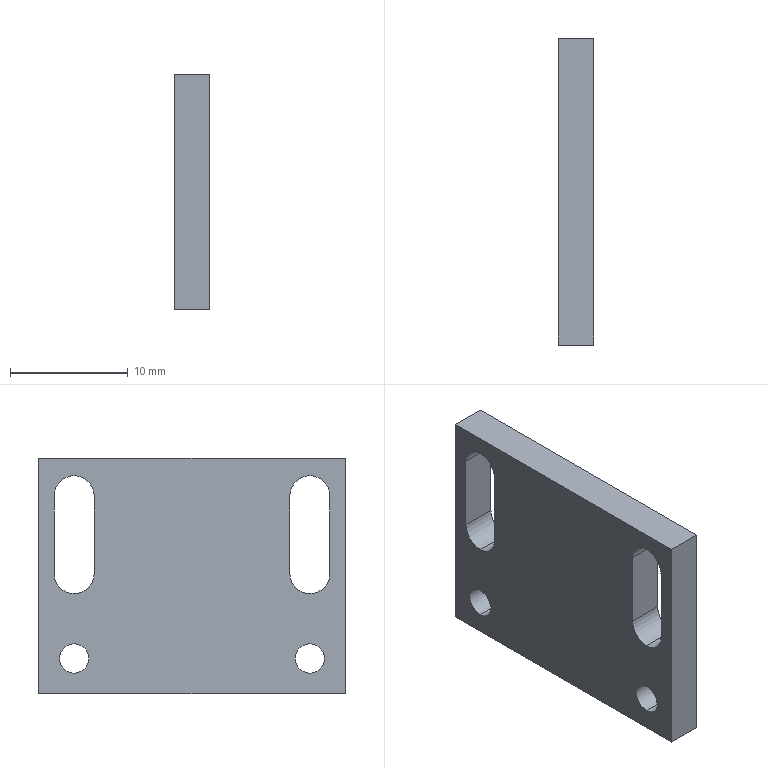Part | NX | features BREP 1 | 1 solid | 20 faces | box 3 x 26 x 20 mm | volume 1341 mm3 | plane 10 | cylinder 10 | commonest cylinder face diameters 3.4 x6 2.5 x4
STEP:
#1=CARTESIAN_POINT('',(3.,11.7,6.8));
#2=VERTEX_POINT('',#1);
#3=CARTESIAN_POINT('',(0.,11.7,6.8));
#4=VERTEX_POINT('',#3);
#5=CARTESIAN_POINT('',(0.,11.7,6.8));
#6=DIRECTION('',(-1.,0.,0.));
#7=VECTOR('',#6,1000.);
#8=LINE('',#5,#7);
#9=EDGE_CURVE('',#2,#4,#8,.T.);
#10=ORIENTED_EDGE('',*,*,#9,.T.);
#11=CARTESIAN_POINT('',(0.,11.7,0.2));
#12=VERTEX_POINT('',#11);
#13=CARTESIAN_POINT('',(0.,11.7,0.2));
#14=DIRECTION('',(0.,0.,1.));
#15=VECTOR('',#14,1000.);
#16=LINE('',#13,#15);
#17=EDGE_CURVE('',#12,#4,#16,.T.);
#18=ORIENTED_EDGE('',*,*,#17,.F.);
#19=CARTESIAN_POINT('',(3.,11.7,0.2));
#20=VERTEX_POINT('',#19);
#21=CARTESIAN_POINT('',(0.,11.7,0.2));
#22=DIRECTION('',(-1.,0.,0.));
#23=VECTOR('',#22,1000.);
#24=LINE('',#21,#23);
#25=EDGE_CURVE('',#20,#12,#24,.T.);
#26=ORIENTED_EDGE('',*,*,#25,.F.);
#27=CARTESIAN_POINT('',(3.,11.7,0.2));
#28=DIRECTION('',(0.,0.,1.));
#29=VECTOR('',#28,1000.);
#30=LINE('',#27,#29);
#31=EDGE_CURVE('',#20,#2,#30,.T.);
#32=ORIENTED_EDGE('',*,*,#31,.T.);
#33=EDGE_LOOP('',(#10,#18,#26,#32));
#34=FACE_BOUND('',#33,.T.);
#35=CARTESIAN_POINT('',(0.,11.7,0.2));
#36=DIRECTION('',(0.,1.,0.));
#37=DIRECTION('',(-1.,0.,0.));
#38=AXIS2_PLACEMENT_3D('',#35,#36,#37);
#39=PLANE('',#38);
#40=ADVANCED_FACE('',(#34),#39,.F.);
#41=CARTESIAN_POINT('',(0.,8.3,6.8));
#42=VERTEX_POINT('',#41);
#43=CARTESIAN_POINT('',(3.,8.3,6.8));
#44=VERTEX_POINT('',#43);
#45=CARTESIAN_POINT('',(3.,8.3,6.8));
#46=DIRECTION('',(1.,0.,0.));
#47=VECTOR('',#46,1000.);
#48=LINE('',#45,#47);
#49=EDGE_CURVE('',#42,#44,#48,.T.);
#50=ORIENTED_EDGE('',*,*,#49,.T.);
#51=CARTESIAN_POINT('',(3.,8.3,0.2));
#52=VERTEX_POINT('',#51);
#53=CARTESIAN_POINT('',(3.,8.3,0.2));
#54=DIRECTION('',(0.,0.,1.));
#55=VECTOR('',#54,1000.);
#56=LINE('',#53,#55);
#57=EDGE_CURVE('',#52,#44,#56,.T.);
#58=ORIENTED_EDGE('',*,*,#57,.F.);
#59=CARTESIAN_POINT('',(0.,8.3,0.2));
#60=VERTEX_POINT('',#59);
#61=CARTESIAN_POINT('',(3.,8.3,0.2));
#62=DIRECTION('',(-1.,0.,0.));
#63=VECTOR('',#62,1000.);
#64=LINE('',#61,#63);
#65=EDGE_CURVE('',#52,#60,#64,.T.);
#66=ORIENTED_EDGE('',*,*,#65,.T.);
#67=CARTESIAN_POINT('',(0.,8.3,0.2));
#68=DIRECTION('',(0.,0.,1.));
#69=VECTOR('',#68,1000.);
#70=LINE('',#67,#69);
#71=EDGE_CURVE('',#60,#42,#70,.T.);
#72=ORIENTED_EDGE('',*,*,#71,.T.);
#73=EDGE_LOOP('',(#50,#58,#66,#72));
#74=FACE_BOUND('',#73,.T.);
#75=CARTESIAN_POINT('',(3.,8.3,0.2));
#76=DIRECTION('',(0.,-1.,0.));
#77=DIRECTION('',(0.,0.,-1.));
#78=AXIS2_PLACEMENT_3D('',#75,#76,#77);
#79=PLANE('',#78);
#80=ADVANCED_FACE('',(#74),#79,.F.);
#81=CARTESIAN_POINT('',(0.,10.,-1.5));
#82=VERTEX_POINT('',#81);
#83=CARTESIAN_POINT('',(3.,10.,-1.5));
#84=VERTEX_POINT('',#83);
#85=CARTESIAN_POINT('',(3.,10.,-1.5));
#86=DIRECTION('',(1.,0.,0.));
#87=VECTOR('',#86,1000.);
#88=LINE('',#85,#87);
#89=EDGE_CURVE('',#82,#84,#88,.T.);
#90=ORIENTED_EDGE('',*,*,#89,.F.);
#91=CARTESIAN_POINT('',(0.,10.,0.2));
#92=DIRECTION('',(1.,0.,0.));
#93=DIRECTION('',(0.,0.,-1.));
#94=AXIS2_PLACEMENT_3D('',#91,#92,#93);
#95=CIRCLE('',#94,1.7);
#96=EDGE_CURVE('',#60,#82,#95,.T.);
#97=ORIENTED_EDGE('',*,*,#96,.F.);
#98=ORIENTED_EDGE('',*,*,#65,.F.);
#99=CARTESIAN_POINT('',(3.,10.,0.2));
#100=DIRECTION('',(1.,0.,0.));
#101=DIRECTION('',(0.,0.,-1.));
#102=AXIS2_PLACEMENT_3D('',#99,#100,#101);
#103=CIRCLE('',#102,1.7);
#104=EDGE_CURVE('',#52,#84,#103,.T.);
#105=ORIENTED_EDGE('',*,*,#104,.T.);
#106=EDGE_LOOP('',(#90,#97,#98,#105));
#107=FACE_BOUND('',#106,.T.);
#108=CARTESIAN_POINT('',(3.,10.,0.2));
#109=DIRECTION('',(1.,0.,0.));
#110=DIRECTION('',(0.,0.,-1.));
#111=AXIS2_PLACEMENT_3D('',#108,#109,#110);
#112=CYLINDRICAL_SURFACE('',#111,1.7);
#113=ADVANCED_FACE('',(#107),#112,.F.);
#114=CARTESIAN_POINT('',(0.,10.,6.8));
#115=DIRECTION('',(1.,0.,0.));
#116=DIRECTION('',(0.,0.,-1.));
#117=AXIS2_PLACEMENT_3D('',#114,#115,#116);
#118=CIRCLE('',#117,1.7);
#119=EDGE_CURVE('',#4,#42,#118,.T.);
#120=ORIENTED_EDGE('',*,*,#119,.F.);
#121=ORIENTED_EDGE('',*,*,#9,.F.);
#122=CARTESIAN_POINT('',(3.,10.,6.8));
#123=DIRECTION('',(1.,0.,0.));
#124=DIRECTION('',(0.,0.,-1.));
#125=AXIS2_PLACEMENT_3D('',#122,#123,#124);
#126=CIRCLE('',#125,1.7);
#127=EDGE_CURVE('',#2,#44,#126,.T.);
#128=ORIENTED_EDGE('',*,*,#127,.T.);
#129=ORIENTED_EDGE('',*,*,#49,.F.);
#130=EDGE_LOOP('',(#120,#121,#128,#129));
#131=FACE_BOUND('',#130,.T.);
#132=CARTESIAN_POINT('',(3.,10.,6.8));
#133=DIRECTION('',(1.,0.,0.));
#134=DIRECTION('',(0.,0.,-1.));
#135=AXIS2_PLACEMENT_3D('',#132,#133,#134);
#136=CYLINDRICAL_SURFACE('',#135,1.7);
#137=ADVANCED_FACE('',(#131),#136,.F.);
#138=CARTESIAN_POINT('',(3.,-8.3,6.8));
#139=VERTEX_POINT('',#138);
#140=CARTESIAN_POINT('',(0.,-8.3,6.8));
#141=VERTEX_POINT('',#140);
#142=CARTESIAN_POINT('',(0.,-8.3,6.8));
#143=DIRECTION('',(-1.,0.,0.));
#144=VECTOR('',#143,1000.);
#145=LINE('',#142,#144);
#146=EDGE_CURVE('',#139,#141,#145,.T.);
#147=ORIENTED_EDGE('',*,*,#146,.T.);
#148=CARTESIAN_POINT('',(0.,-8.3,0.2));
#149=VERTEX_POINT('',#148);
#150=CARTESIAN_POINT('',(0.,-8.3,0.2));
#151=DIRECTION('',(0.,0.,1.));
#152=VECTOR('',#151,1000.);
#153=LINE('',#150,#152);
#154=EDGE_CURVE('',#149,#141,#153,.T.);
#155=ORIENTED_EDGE('',*,*,#154,.F.);
#156=CARTESIAN_POINT('',(3.,-8.3,0.2));
#157=VERTEX_POINT('',#156);
#158=CARTESIAN_POINT('',(0.,-8.3,0.2));
#159=DIRECTION('',(-1.,0.,0.));
#160=VECTOR('',#159,1000.);
#161=LINE('',#158,#160);
#162=EDGE_CURVE('',#157,#149,#161,.T.);
#163=ORIENTED_EDGE('',*,*,#162,.F.);
#164=CARTESIAN_POINT('',(3.,-8.3,0.2));
#165=DIRECTION('',(0.,0.,1.));
#166=VECTOR('',#165,1000.);
#167=LINE('',#164,#166);
#168=EDGE_CURVE('',#157,#139,#167,.T.);
#169=ORIENTED_EDGE('',*,*,#168,.T.);
#170=EDGE_LOOP('',(#147,#155,#163,#169));
#171=FACE_BOUND('',#170,.T.);
#172=CARTESIAN_POINT('',(0.,-8.3,0.2));
#173=DIRECTION('',(0.,1.,0.));
#174=DIRECTION('',(-1.,0.,0.));
#175=AXIS2_PLACEMENT_3D('',#172,#173,#174);
#176=PLANE('',#175);
#177=ADVANCED_FACE('',(#171),#176,.F.);
#178=CARTESIAN_POINT('',(0.,-11.7,6.8));
#179=VERTEX_POINT('',#178);
#180=CARTESIAN_POINT('',(3.,-11.7,6.8));
#181=VERTEX_POINT('',#180);
#182=CARTESIAN_POINT('',(3.,-11.7,6.8));
#183=DIRECTION('',(1.,0.,0.));
#184=VECTOR('',#183,1000.);
#185=LINE('',#182,#184);
#186=EDGE_CURVE('',#179,#181,#185,.T.);
#187=ORIENTED_EDGE('',*,*,#186,.T.);
#188=CARTESIAN_POINT('',(3.,-11.7,0.2));
#189=VERTEX_POINT('',#188);
#190=CARTESIAN_POINT('',(3.,-11.7,0.2));
#191=DIRECTION('',(0.,0.,1.));
#192=VECTOR('',#191,1000.);
#193=LINE('',#190,#192);
#194=EDGE_CURVE('',#189,#181,#193,.T.);
#195=ORIENTED_EDGE('',*,*,#194,.F.);
#196=CARTESIAN_POINT('',(0.,-11.7,0.2));
#197=VERTEX_POINT('',#196);
#198=CARTESIAN_POINT('',(3.,-11.7,0.2));
#199=DIRECTION('',(-1.,0.,0.));
#200=VECTOR('',#199,1000.);
#201=LINE('',#198,#200);
#202=EDGE_CURVE('',#189,#197,#201,.T.);
#203=ORIENTED_EDGE('',*,*,#202,.T.);
#204=CARTESIAN_POINT('',(0.,-11.7,0.2));
#205=DIRECTION('',(0.,0.,1.));
#206=VECTOR('',#205,1000.);
#207=LINE('',#204,#206);
#208=EDGE_CURVE('',#197,#179,#207,.T.);
#209=ORIENTED_EDGE('',*,*,#208,.T.);
#210=EDGE_LOOP('',(#187,#195,#203,#209));
#211=FACE_BOUND('',#210,.T.);
#212=CARTESIAN_POINT('',(3.,-11.7,0.2));
#213=DIRECTION('',(0.,-1.,0.));
#214=DIRECTION('',(0.,0.,-1.));
#215=AXIS2_PLACEMENT_3D('',#212,#213,#214);
#216=PLANE('',#215);
#217=ADVANCED_FACE('',(#211),#216,.F.);
#218=CARTESIAN_POINT('',(0.,-10.,-1.5));
#219=VERTEX_POINT('',#218);
#220=CARTESIAN_POINT('',(3.,-10.,-1.5));
#221=VERTEX_POINT('',#220);
#222=CARTESIAN_POINT('',(3.,-10.,-1.5));
#223=DIRECTION('',(1.,0.,0.));
#224=VECTOR('',#223,1000.);
#225=LINE('',#222,#224);
#226=EDGE_CURVE('',#219,#221,#225,.T.);
#227=ORIENTED_EDGE('',*,*,#226,.F.);
#228=CARTESIAN_POINT('',(0.,-10.,0.2));
#229=DIRECTION('',(1.,0.,0.));
#230=DIRECTION('',(0.,0.,-1.));
#231=AXIS2_PLACEMENT_3D('',#228,#229,#230);
#232=CIRCLE('',#231,1.7);
#233=EDGE_CURVE('',#197,#219,#232,.T.);
#234=ORIENTED_EDGE('',*,*,#233,.F.);
#235=ORIENTED_EDGE('',*,*,#202,.F.);
#236=CARTESIAN_POINT('',(3.,-10.,0.2));
#237=DIRECTION('',(1.,0.,0.));
#238=DIRECTION('',(0.,0.,-1.));
#239=AXIS2_PLACEMENT_3D('',#236,#237,#238);
#240=CIRCLE('',#239,1.7);
#241=EDGE_CURVE('',#189,#221,#240,.T.);
#242=ORIENTED_EDGE('',*,*,#241,.T.);
#243=EDGE_LOOP('',(#227,#234,#235,#242));
#244=FACE_BOUND('',#243,.T.);
#245=CARTESIAN_POINT('',(3.,-10.,0.2));
#246=DIRECTION('',(1.,0.,0.));
#247=DIRECTION('',(0.,0.,-1.));
#248=AXIS2_PLACEMENT_3D('',#245,#246,#247);
#249=CYLINDRICAL_SURFACE('',#248,1.7);
#250=ADVANCED_FACE('',(#244),#249,.F.);
#251=CARTESIAN_POINT('',(0.,-10.,6.8));
#252=DIRECTION('',(1.,0.,0.));
#253=DIRECTION('',(0.,0.,-1.));
#254=AXIS2_PLACEMENT_3D('',#251,#252,#253);
#255=CIRCLE('',#254,1.7);
#256=EDGE_CURVE('',#141,#179,#255,.T.);
#257=ORIENTED_EDGE('',*,*,#256,.F.);
#258=ORIENTED_EDGE('',*,*,#146,.F.);
#259=CARTESIAN_POINT('',(3.,-10.,6.8));
#260=DIRECTION('',(1.,0.,0.));
#261=DIRECTION('',(0.,0.,-1.));
#262=AXIS2_PLACEMENT_3D('',#259,#260,#261);
#263=CIRCLE('',#262,1.7);
#264=EDGE_CURVE('',#139,#181,#263,.T.);
#265=ORIENTED_EDGE('',*,*,#264,.T.);
#266=ORIENTED_EDGE('',*,*,#186,.F.);
#267=EDGE_LOOP('',(#257,#258,#265,#266));
#268=FACE_BOUND('',#267,.T.);
#269=CARTESIAN_POINT('',(3.,-10.,6.8));
#270=DIRECTION('',(1.,0.,0.));
#271=DIRECTION('',(0.,0.,-1.));
#272=AXIS2_PLACEMENT_3D('',#269,#270,#271);
#273=CYLINDRICAL_SURFACE('',#272,1.7);
#274=ADVANCED_FACE('',(#268),#273,.F.);
#275=CARTESIAN_POINT('',(0.,10.,-5.75));
#276=VERTEX_POINT('',#275);
#277=CARTESIAN_POINT('',(3.,10.,-5.75));
#278=VERTEX_POINT('',#277);
#279=CARTESIAN_POINT('',(3.,10.,-5.75));
#280=DIRECTION('',(1.,0.,0.));
#281=VECTOR('',#280,1000.);
#282=LINE('',#279,#281);
#283=EDGE_CURVE('',#276,#278,#282,.T.);
#284=ORIENTED_EDGE('',*,*,#283,.F.);
#285=CARTESIAN_POINT('',(0.,10.,-8.25));
#286=VERTEX_POINT('',#285);
#287=CARTESIAN_POINT('',(0.,10.,-7.));
#288=DIRECTION('',(-1.,0.,0.));
#289=DIRECTION('',(0.,0.,1.));
#290=AXIS2_PLACEMENT_3D('',#287,#288,#289);
#291=CIRCLE('',#290,1.25);
#292=EDGE_CURVE('',#276,#286,#291,.T.);
#293=ORIENTED_EDGE('',*,*,#292,.T.);
#294=CARTESIAN_POINT('',(3.,10.,-8.25));
#295=VERTEX_POINT('',#294);
#296=CARTESIAN_POINT('',(3.,10.,-8.25));
#297=DIRECTION('',(1.,0.,0.));
#298=VECTOR('',#297,1000.);
#299=LINE('',#296,#298);
#300=EDGE_CURVE('',#286,#295,#299,.T.);
#301=ORIENTED_EDGE('',*,*,#300,.T.);
#302=CARTESIAN_POINT('',(3.,10.,-7.));
#303=DIRECTION('',(1.,0.,0.));
#304=DIRECTION('',(0.,0.,-1.));
#305=AXIS2_PLACEMENT_3D('',#302,#303,#304);
#306=CIRCLE('',#305,1.25);
#307=EDGE_CURVE('',#295,#278,#306,.T.);
#308=ORIENTED_EDGE('',*,*,#307,.T.);
#309=EDGE_LOOP('',(#284,#293,#301,#308));
#310=FACE_BOUND('',#309,.T.);
#311=CARTESIAN_POINT('',(3.,10.,-7.));
#312=DIRECTION('',(1.,0.,0.));
#313=DIRECTION('',(0.,0.,-1.));
#314=AXIS2_PLACEMENT_3D('',#311,#312,#313);
#315=CYLINDRICAL_SURFACE('',#314,1.25);
#316=ADVANCED_FACE('',(#310),#315,.F.);
#317=CARTESIAN_POINT('',(0.,-10.,-5.75));
#318=VERTEX_POINT('',#317);
#319=CARTESIAN_POINT('',(3.,-10.,-5.75));
#320=VERTEX_POINT('',#319);
#321=CARTESIAN_POINT('',(3.,-10.,-5.75));
#322=DIRECTION('',(1.,0.,0.));
#323=VECTOR('',#322,1000.);
#324=LINE('',#321,#323);
#325=EDGE_CURVE('',#318,#320,#324,.T.);
#326=ORIENTED_EDGE('',*,*,#325,.F.);
#327=CARTESIAN_POINT('',(0.,-10.,-8.25));
#328=VERTEX_POINT('',#327);
#329=CARTESIAN_POINT('',(0.,-10.,-7.));
#330=DIRECTION('',(-1.,0.,0.));
#331=DIRECTION('',(0.,0.,1.));
#332=AXIS2_PLACEMENT_3D('',#329,#330,#331);
#333=CIRCLE('',#332,1.25);
#334=EDGE_CURVE('',#318,#328,#333,.T.);
#335=ORIENTED_EDGE('',*,*,#334,.T.);
#336=CARTESIAN_POINT('',(3.,-10.,-8.25));
#337=VERTEX_POINT('',#336);
#338=CARTESIAN_POINT('',(3.,-10.,-8.25));
#339=DIRECTION('',(1.,0.,0.));
#340=VECTOR('',#339,1000.);
#341=LINE('',#338,#340);
#342=EDGE_CURVE('',#328,#337,#341,.T.);
#343=ORIENTED_EDGE('',*,*,#342,.T.);
#344=CARTESIAN_POINT('',(3.,-10.,-7.));
#345=DIRECTION('',(1.,0.,0.));
#346=DIRECTION('',(0.,0.,-1.));
#347=AXIS2_PLACEMENT_3D('',#344,#345,#346);
#348=CIRCLE('',#347,1.25);
#349=EDGE_CURVE('',#337,#320,#348,.T.);
#350=ORIENTED_EDGE('',*,*,#349,.T.);
#351=EDGE_LOOP('',(#326,#335,#343,#350));
#352=FACE_BOUND('',#351,.T.);
#353=CARTESIAN_POINT('',(3.,-10.,-7.));
#354=DIRECTION('',(1.,0.,0.));
#355=DIRECTION('',(0.,0.,-1.));
#356=AXIS2_PLACEMENT_3D('',#353,#354,#355);
#357=CYLINDRICAL_SURFACE('',#356,1.25);
#358=ADVANCED_FACE('',(#352),#357,.F.);
#359=CARTESIAN_POINT('',(0.,-13.,10.));
#360=VERTEX_POINT('',#359);
#361=CARTESIAN_POINT('',(0.,-13.,-10.));
#362=VERTEX_POINT('',#361);
#363=CARTESIAN_POINT('',(0.,-13.,10.));
#364=DIRECTION('',(0.,0.,-1.));
#365=VECTOR('',#364,1000.);
#366=LINE('',#363,#365);
#367=EDGE_CURVE('',#360,#362,#366,.T.);
#368=ORIENTED_EDGE('',*,*,#367,.T.);
#369=CARTESIAN_POINT('',(3.,-13.,-10.));
#370=VERTEX_POINT('',#369);
#371=CARTESIAN_POINT('',(3.,-13.,-10.));
#372=DIRECTION('',(-1.,0.,0.));
#373=VECTOR('',#372,1000.);
#374=LINE('',#371,#373);
#375=EDGE_CURVE('',#370,#362,#374,.T.);
#376=ORIENTED_EDGE('',*,*,#375,.F.);
#377=CARTESIAN_POINT('',(3.,-13.,10.));
#378=VERTEX_POINT('',#377);
#379=CARTESIAN_POINT('',(3.,-13.,10.));
#380=DIRECTION('',(0.,0.,-1.));
#381=VECTOR('',#380,1000.);
#382=LINE('',#379,#381);
#383=EDGE_CURVE('',#378,#370,#382,.T.);
#384=ORIENTED_EDGE('',*,*,#383,.F.);
#385=CARTESIAN_POINT('',(3.,-13.,10.));
#386=DIRECTION('',(-1.,0.,0.));
#387=VECTOR('',#386,1000.);
#388=LINE('',#385,#387);
#389=EDGE_CURVE('',#378,#360,#388,.T.);
#390=ORIENTED_EDGE('',*,*,#389,.T.);
#391=EDGE_LOOP('',(#368,#376,#384,#390));
#392=FACE_BOUND('',#391,.T.);
#393=CARTESIAN_POINT('',(3.,-13.,10.));
#394=DIRECTION('',(0.,1.,0.));
#395=DIRECTION('',(0.,0.,1.));
#396=AXIS2_PLACEMENT_3D('',#393,#394,#395);
#397=PLANE('',#396);
#398=ADVANCED_FACE('',(#392),#397,.F.);
#399=CARTESIAN_POINT('',(0.,13.,10.));
#400=VERTEX_POINT('',#399);
#401=CARTESIAN_POINT('',(0.,-13.,10.));
#402=DIRECTION('',(0.,-1.,0.));
#403=VECTOR('',#402,1000.);
#404=LINE('',#401,#403);
#405=EDGE_CURVE('',#400,#360,#404,.T.);
#406=ORIENTED_EDGE('',*,*,#405,.T.);
#407=ORIENTED_EDGE('',*,*,#389,.F.);
#408=CARTESIAN_POINT('',(3.,13.,10.));
#409=VERTEX_POINT('',#408);
#410=CARTESIAN_POINT('',(3.,-13.,10.));
#411=DIRECTION('',(0.,-1.,0.));
#412=VECTOR('',#411,1000.);
#413=LINE('',#410,#412);
#414=EDGE_CURVE('',#409,#378,#413,.T.);
#415=ORIENTED_EDGE('',*,*,#414,.F.);
#416=CARTESIAN_POINT('',(3.,13.,10.));
#417=DIRECTION('',(-1.,0.,0.));
#418=VECTOR('',#417,1000.);
#419=LINE('',#416,#418);
#420=EDGE_CURVE('',#409,#400,#419,.T.);
#421=ORIENTED_EDGE('',*,*,#420,.T.);
#422=EDGE_LOOP('',(#406,#407,#415,#421));
#423=FACE_BOUND('',#422,.T.);
#424=CARTESIAN_POINT('',(3.,-13.,10.));
#425=DIRECTION('',(0.,0.,-1.));
#426=DIRECTION('',(-1.,0.,0.));
#427=AXIS2_PLACEMENT_3D('',#424,#425,#426);
#428=PLANE('',#427);
#429=ADVANCED_FACE('',(#423),#428,.F.);
#430=CARTESIAN_POINT('',(0.,13.,-10.));
#431=VERTEX_POINT('',#430);
#432=CARTESIAN_POINT('',(0.,13.,10.));
#433=DIRECTION('',(0.,0.,1.));
#434=VECTOR('',#433,1000.);
#435=LINE('',#432,#434);
#436=EDGE_CURVE('',#431,#400,#435,.T.);
#437=ORIENTED_EDGE('',*,*,#436,.T.);
#438=ORIENTED_EDGE('',*,*,#420,.F.);
#439=CARTESIAN_POINT('',(3.,13.,-10.));
#440=VERTEX_POINT('',#439);
#441=CARTESIAN_POINT('',(3.,13.,10.));
#442=DIRECTION('',(0.,0.,1.));
#443=VECTOR('',#442,1000.);
#444=LINE('',#441,#443);
#445=EDGE_CURVE('',#440,#409,#444,.T.);
#446=ORIENTED_EDGE('',*,*,#445,.F.);
#447=CARTESIAN_POINT('',(3.,13.,-10.));
#448=DIRECTION('',(-1.,0.,0.));
#449=VECTOR('',#448,1000.);
#450=LINE('',#447,#449);
#451=EDGE_CURVE('',#440,#431,#450,.T.);
#452=ORIENTED_EDGE('',*,*,#451,.T.);
#453=EDGE_LOOP('',(#437,#438,#446,#452));
#454=FACE_BOUND('',#453,.T.);
#455=CARTESIAN_POINT('',(3.,13.,10.));
#456=DIRECTION('',(0.,-1.,0.));
#457=DIRECTION('',(0.,0.,-1.));
#458=AXIS2_PLACEMENT_3D('',#455,#456,#457);
#459=PLANE('',#458);
#460=ADVANCED_FACE('',(#454),#459,.F.);
#461=CARTESIAN_POINT('',(0.,-13.,-10.));
#462=DIRECTION('',(0.,1.,0.));
#463=VECTOR('',#462,1000.);
#464=LINE('',#461,#463);
#465=EDGE_CURVE('',#362,#431,#464,.T.);
#466=ORIENTED_EDGE('',*,*,#465,.T.);
#467=ORIENTED_EDGE('',*,*,#451,.F.);
#468=CARTESIAN_POINT('',(3.,-13.,-10.));
#469=DIRECTION('',(0.,1.,0.));
#470=VECTOR('',#469,1000.);
#471=LINE('',#468,#470);
#472=EDGE_CURVE('',#370,#440,#471,.T.);
#473=ORIENTED_EDGE('',*,*,#472,.F.);
#474=ORIENTED_EDGE('',*,*,#375,.T.);
#475=EDGE_LOOP('',(#466,#467,#473,#474));
#476=FACE_BOUND('',#475,.T.);
#477=CARTESIAN_POINT('',(3.,-13.,-10.));
#478=DIRECTION('',(0.,0.,1.));
#479=DIRECTION('',(1.,0.,0.));
#480=AXIS2_PLACEMENT_3D('',#477,#478,#479);
#481=PLANE('',#480);
#482=ADVANCED_FACE('',(#476),#481,.F.);
#483=ORIENTED_EDGE('',*,*,#31,.F.);
#484=CARTESIAN_POINT('',(3.,10.,0.2));
#485=DIRECTION('',(1.,0.,0.));
#486=DIRECTION('',(0.,0.,-1.));
#487=AXIS2_PLACEMENT_3D('',#484,#485,#486);
#488=CIRCLE('',#487,1.7);
#489=EDGE_CURVE('',#84,#20,#488,.T.);
#490=ORIENTED_EDGE('',*,*,#489,.F.);
#491=ORIENTED_EDGE('',*,*,#104,.F.);
#492=ORIENTED_EDGE('',*,*,#57,.T.);
#493=ORIENTED_EDGE('',*,*,#127,.F.);
#494=EDGE_LOOP('',(#483,#490,#491,#492,#493));
#495=FACE_BOUND('',#494,.T.);
#496=ORIENTED_EDGE('',*,*,#264,.F.);
#497=ORIENTED_EDGE('',*,*,#168,.F.);
#498=CARTESIAN_POINT('',(3.,-10.,0.2));
#499=DIRECTION('',(1.,0.,0.));
#500=DIRECTION('',(0.,0.,-1.));
#501=AXIS2_PLACEMENT_3D('',#498,#499,#500);
#502=CIRCLE('',#501,1.7);
#503=EDGE_CURVE('',#221,#157,#502,.T.);
#504=ORIENTED_EDGE('',*,*,#503,.F.);
#505=ORIENTED_EDGE('',*,*,#241,.F.);
#506=ORIENTED_EDGE('',*,*,#194,.T.);
#507=EDGE_LOOP('',(#496,#497,#504,#505,#506));
#508=FACE_BOUND('',#507,.T.);
#509=ORIENTED_EDGE('',*,*,#307,.F.);
#510=CARTESIAN_POINT('',(3.,10.,-7.));
#511=DIRECTION('',(1.,0.,0.));
#512=DIRECTION('',(0.,0.,-1.));
#513=AXIS2_PLACEMENT_3D('',#510,#511,#512);
#514=CIRCLE('',#513,1.25);
#515=EDGE_CURVE('',#278,#295,#514,.T.);
#516=ORIENTED_EDGE('',*,*,#515,.F.);
#517=EDGE_LOOP('',(#509,#516));
#518=FACE_BOUND('',#517,.T.);
#519=ORIENTED_EDGE('',*,*,#349,.F.);
#520=CARTESIAN_POINT('',(3.,-10.,-7.));
#521=DIRECTION('',(1.,0.,0.));
#522=DIRECTION('',(0.,0.,-1.));
#523=AXIS2_PLACEMENT_3D('',#520,#521,#522);
#524=CIRCLE('',#523,1.25);
#525=EDGE_CURVE('',#320,#337,#524,.T.);
#526=ORIENTED_EDGE('',*,*,#525,.F.);
#527=EDGE_LOOP('',(#519,#526));
#528=FACE_BOUND('',#527,.T.);
#529=ORIENTED_EDGE('',*,*,#472,.T.);
#530=ORIENTED_EDGE('',*,*,#445,.T.);
#531=ORIENTED_EDGE('',*,*,#414,.T.);
#532=ORIENTED_EDGE('',*,*,#383,.T.);
#533=EDGE_LOOP('',(#529,#530,#531,#532));
#534=FACE_BOUND('',#533,.T.);
#535=CARTESIAN_POINT('',(3.,0.,0.));
#536=DIRECTION('',(-1.,0.,0.));
#537=DIRECTION('',(0.,0.,1.));
#538=AXIS2_PLACEMENT_3D('',#535,#536,#537);
#539=PLANE('',#538);
#540=ADVANCED_FACE('',(#495,#508,#518,#528,#534),#539,.F.);
#541=ORIENTED_EDGE('',*,*,#17,.T.);
#542=ORIENTED_EDGE('',*,*,#119,.T.);
#543=ORIENTED_EDGE('',*,*,#71,.F.);
#544=ORIENTED_EDGE('',*,*,#96,.T.);
#545=CARTESIAN_POINT('',(0.,10.,0.2));
#546=DIRECTION('',(1.,0.,0.));
#547=DIRECTION('',(0.,0.,-1.));
#548=AXIS2_PLACEMENT_3D('',#545,#546,#547);
#549=CIRCLE('',#548,1.7);
#550=EDGE_CURVE('',#82,#12,#549,.T.);
#551=ORIENTED_EDGE('',*,*,#550,.T.);
#552=EDGE_LOOP('',(#541,#542,#543,#544,#551));
#553=FACE_BOUND('',#552,.T.);
#554=ORIENTED_EDGE('',*,*,#233,.T.);
#555=CARTESIAN_POINT('',(0.,-10.,0.2));
#556=DIRECTION('',(1.,0.,0.));
#557=DIRECTION('',(0.,0.,-1.));
#558=AXIS2_PLACEMENT_3D('',#555,#556,#557);
#559=CIRCLE('',#558,1.7);
#560=EDGE_CURVE('',#219,#149,#559,.T.);
#561=ORIENTED_EDGE('',*,*,#560,.T.);
#562=ORIENTED_EDGE('',*,*,#154,.T.);
#563=ORIENTED_EDGE('',*,*,#256,.T.);
#564=ORIENTED_EDGE('',*,*,#208,.F.);
#565=EDGE_LOOP('',(#554,#561,#562,#563,#564));
#566=FACE_BOUND('',#565,.T.);
#567=ORIENTED_EDGE('',*,*,#465,.F.);
#568=ORIENTED_EDGE('',*,*,#367,.F.);
#569=ORIENTED_EDGE('',*,*,#405,.F.);
#570=ORIENTED_EDGE('',*,*,#436,.F.);
#571=EDGE_LOOP('',(#567,#568,#569,#570));
#572=FACE_BOUND('',#571,.T.);
#573=CARTESIAN_POINT('',(0.,-10.,-7.));
#574=DIRECTION('',(-1.,0.,0.));
#575=DIRECTION('',(0.,0.,1.));
#576=AXIS2_PLACEMENT_3D('',#573,#574,#575);
#577=CIRCLE('',#576,1.25);
#578=EDGE_CURVE('',#328,#318,#577,.T.);
#579=ORIENTED_EDGE('',*,*,#578,.F.);
#580=ORIENTED_EDGE('',*,*,#334,.F.);
#581=EDGE_LOOP('',(#579,#580));
#582=FACE_BOUND('',#581,.T.);
#583=CARTESIAN_POINT('',(0.,10.,-7.));
#584=DIRECTION('',(-1.,0.,0.));
#585=DIRECTION('',(0.,0.,1.));
#586=AXIS2_PLACEMENT_3D('',#583,#584,#585);
#587=CIRCLE('',#586,1.25);
#588=EDGE_CURVE('',#286,#276,#587,.T.);
#589=ORIENTED_EDGE('',*,*,#588,.F.);
#590=ORIENTED_EDGE('',*,*,#292,.F.);
#591=EDGE_LOOP('',(#589,#590));
#592=FACE_BOUND('',#591,.T.);
#593=CARTESIAN_POINT('',(0.,0.,0.));
#594=DIRECTION('',(-1.,0.,0.));
#595=DIRECTION('',(0.,0.,1.));
#596=AXIS2_PLACEMENT_3D('',#593,#594,#595);
#597=PLANE('',#596);
#598=ADVANCED_FACE('',(#553,#566,#572,#582,#592),#597,.T.);
#599=ORIENTED_EDGE('',*,*,#578,.T.);
#600=ORIENTED_EDGE('',*,*,#325,.T.);
#601=ORIENTED_EDGE('',*,*,#525,.T.);
#602=ORIENTED_EDGE('',*,*,#342,.F.);
#603=EDGE_LOOP('',(#599,#600,#601,#602));
#604=FACE_BOUND('',#603,.T.);
#605=CARTESIAN_POINT('',(3.,-10.,-7.));
#606=DIRECTION('',(1.,0.,0.));
#607=DIRECTION('',(0.,0.,-1.));
#608=AXIS2_PLACEMENT_3D('',#605,#606,#607);
#609=CYLINDRICAL_SURFACE('',#608,1.25);
#610=ADVANCED_FACE('',(#604),#609,.F.);
#611=ORIENTED_EDGE('',*,*,#588,.T.);
#612=ORIENTED_EDGE('',*,*,#283,.T.);
#613=ORIENTED_EDGE('',*,*,#515,.T.);
#614=ORIENTED_EDGE('',*,*,#300,.F.);
#615=EDGE_LOOP('',(#611,#612,#613,#614));
#616=FACE_BOUND('',#615,.T.);
#617=CARTESIAN_POINT('',(3.,10.,-7.));
#618=DIRECTION('',(1.,0.,0.));
#619=DIRECTION('',(0.,0.,-1.));
#620=AXIS2_PLACEMENT_3D('',#617,#618,#619);
#621=CYLINDRICAL_SURFACE('',#620,1.25);
#622=ADVANCED_FACE('',(#616),#621,.F.);
#623=ORIENTED_EDGE('',*,*,#560,.F.);
#624=ORIENTED_EDGE('',*,*,#226,.T.);
#625=ORIENTED_EDGE('',*,*,#503,.T.);
#626=ORIENTED_EDGE('',*,*,#162,.T.);
#627=EDGE_LOOP('',(#623,#624,#625,#626));
#628=FACE_BOUND('',#627,.T.);
#629=CARTESIAN_POINT('',(3.,-10.,0.2));
#630=DIRECTION('',(1.,0.,0.));
#631=DIRECTION('',(0.,0.,-1.));
#632=AXIS2_PLACEMENT_3D('',#629,#630,#631);
#633=CYLINDRICAL_SURFACE('',#632,1.7);
#634=ADVANCED_FACE('',(#628),#633,.F.);
#635=ORIENTED_EDGE('',*,*,#550,.F.);
#636=ORIENTED_EDGE('',*,*,#89,.T.);
#637=ORIENTED_EDGE('',*,*,#489,.T.);
#638=ORIENTED_EDGE('',*,*,#25,.T.);
#639=EDGE_LOOP('',(#635,#636,#637,#638));
#640=FACE_BOUND('',#639,.T.);
#641=CARTESIAN_POINT('',(3.,10.,0.2));
#642=DIRECTION('',(1.,0.,0.));
#643=DIRECTION('',(0.,0.,-1.));
#644=AXIS2_PLACEMENT_3D('',#641,#642,#643);
#645=CYLINDRICAL_SURFACE('',#644,1.7);
#646=ADVANCED_FACE('',(#640),#645,.F.);
#647=CLOSED_SHELL('',(#40,#80,#113,#137,#177,#217,#250,#274,#316,#358,#398,#429,#460,#482,#540,#598,#610,#622,#634,#646));
#648=MANIFOLD_SOLID_BREP('',#647);
#649=(LENGTH_UNIT()NAMED_UNIT(*)SI_UNIT(.MILLI.,.METRE.));
#650=UNCERTAINTY_MEASURE_WITH_UNIT(LENGTH_MEASURE(0.00001),#649,'','');
#651=(NAMED_UNIT(*)PLANE_ANGLE_UNIT()SI_UNIT($,.RADIAN.));
#652=(NAMED_UNIT(*)SI_UNIT($,.STERADIAN.)SOLID_ANGLE_UNIT());
#653=(GEOMETRIC_REPRESENTATION_CONTEXT(3)GLOBAL_UNCERTAINTY_ASSIGNED_CONTEXT((#650))GLOBAL_UNIT_ASSIGNED_CONTEXT((#649,#651,#652))REPRESENTATION_CONTEXT('',''));
#654=ADVANCED_BREP_SHAPE_REPRESENTATION('',(#648),#653);